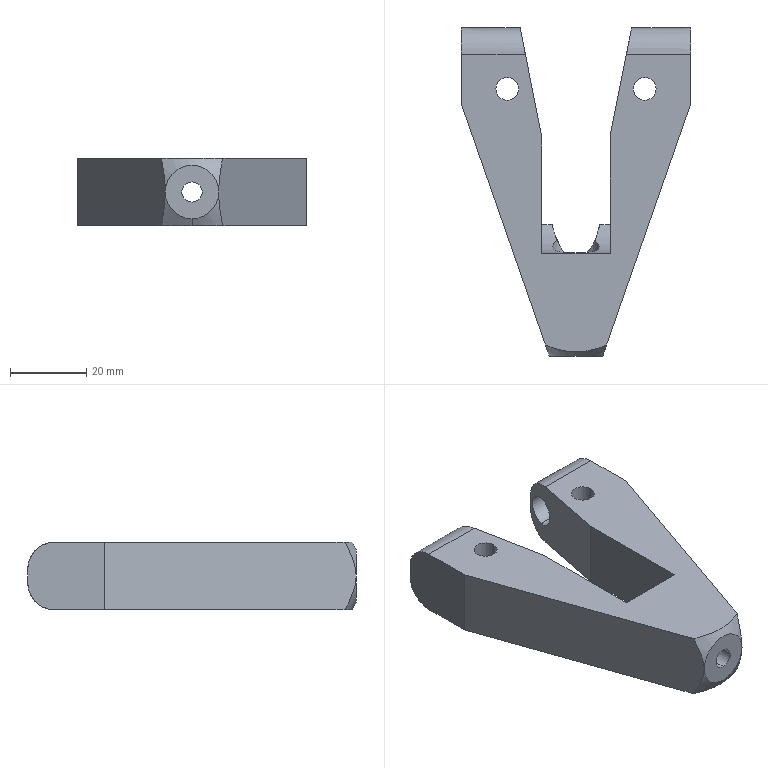Part | SolidWorks | features ICE 5, Extrusion 1, Fillet 1, RevCut 1 | 1 solid | 40 faces | box 60 x 86 x 17.7 mm | volume 37874 mm3 | cylinder 16 | plane 15 | torus 4 | cone 3 | spline 2 | commonest cylinder face diameters 6 x4 8 x4 14 x4 5.3 x2 12.388 x2